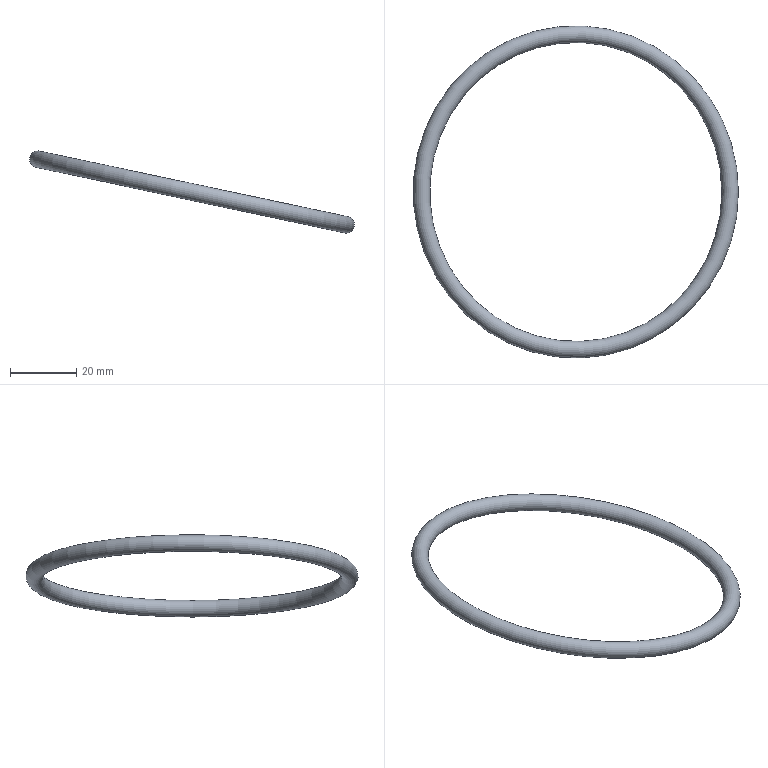Part | STEP file | 8903-010050 (O-ring) | 1 solid | 1 faces | box 97.924 x 100 x 24.752 mm | volume 5860 mm3 | torus 1
STEP:
#1=CARTESIAN_POINT('',(0.,0.,0.));
#2=DIRECTION('',(0.,0.,1.));
#3=DIRECTION('',(1.,0.,0.));
#4=AXIS2_PLACEMENT_3D('',#1,#2,#3);
#5=CARTESIAN_POINT('',(1988.852,-44.547,-308.432));
#6=VERTEX_POINT('',#5);
#7=CARTESIAN_POINT('',(1988.746,-47.045,-308.41));
#8=DIRECTION('',(-0.9772,0.04338,0.2077));
#9=DIRECTION('',(0.04243,0.9991,-0.009019));
#10=AXIS2_PLACEMENT_3D('',#7,#8,#9);
#11=CIRCLE('',#10,2.5);
#12=CARTESIAN_POINT('',(1986.73,-94.5,-307.981));
#13=DIRECTION('',(-0.2079,0.,-0.9781));
#14=DIRECTION('',(0.04243,0.9991,-0.009019));
#15=AXIS2_PLACEMENT_3D('',#12,#13,#14);
#16=TOROIDAL_SURFACE('',#15,47.5,2.5);
#17=CARTESIAN_POINT('',(6.283,0.));
#18=DIRECTION('',(0.,1.));
#19=VECTOR('',#18,1.);
#20=LINE('',#17,#19);
#21=(GEOMETRIC_REPRESENTATION_CONTEXT(2)PARAMETRIC_REPRESENTATION_CONTEXT()REPRESENTATION_CONTEXT('',''));
#22=DEFINITIONAL_REPRESENTATION('',(#20),#21);
#23=PCURVE('',#16,#22);
#24=CARTESIAN_POINT('',(0.,0.));
#25=DIRECTION('',(0.,1.));
#26=VECTOR('',#25,1.);
#27=LINE('',#24,#26);
#28=(GEOMETRIC_REPRESENTATION_CONTEXT(2)PARAMETRIC_REPRESENTATION_CONTEXT()REPRESENTATION_CONTEXT('',''));
#29=DEFINITIONAL_REPRESENTATION('',(#27),#28);
#30=PCURVE('',#16,#29);
#31=SEAM_CURVE('',#11,(#23,#30),.PCURVE_S1.);
#32=EDGE_CURVE('',#6,#6,#31,.T.);
#33=ORIENTED_EDGE('',*,*,#32,.T.);
#34=CARTESIAN_POINT('',(1986.73,-94.5,-307.981));
#35=DIRECTION('',(0.2079,0.,0.9781));
#36=DIRECTION('',(0.04243,0.9991,-0.009019));
#37=AXIS2_PLACEMENT_3D('',#34,#35,#36);
#38=CIRCLE('',#37,50.);
#39=CARTESIAN_POINT('',(6.283,6.283));
#40=DIRECTION('',(-1.,0.));
#41=VECTOR('',#40,1.);
#42=LINE('',#39,#41);
#43=(GEOMETRIC_REPRESENTATION_CONTEXT(2)PARAMETRIC_REPRESENTATION_CONTEXT()REPRESENTATION_CONTEXT('',''));
#44=DEFINITIONAL_REPRESENTATION('',(#42),#43);
#45=PCURVE('',#16,#44);
#46=CARTESIAN_POINT('',(6.283,0.));
#47=DIRECTION('',(-1.,0.));
#48=VECTOR('',#47,1.);
#49=LINE('',#46,#48);
#50=(GEOMETRIC_REPRESENTATION_CONTEXT(2)PARAMETRIC_REPRESENTATION_CONTEXT()REPRESENTATION_CONTEXT('',''));
#51=DEFINITIONAL_REPRESENTATION('',(#49),#50);
#52=PCURVE('',#16,#51);
#53=SEAM_CURVE('',#38,(#45,#52),.PCURVE_S1.);
#54=EDGE_CURVE('',#6,#6,#53,.T.);
#55=ORIENTED_EDGE('',*,*,#54,.T.);
#56=ORIENTED_EDGE('',*,*,#32,.F.);
#57=ORIENTED_EDGE('',*,*,#54,.F.);
#58=EDGE_LOOP('',(#33,#55,#56,#57));
#59=FACE_BOUND('',#58,.T.);
#60=ADVANCED_FACE('',(#59),#16,.T.);
#61=CLOSED_SHELL('',(#60));
#62=MANIFOLD_SOLID_BREP('',#61);
#63=(LENGTH_UNIT()NAMED_UNIT(*)SI_UNIT(.MILLI.,.METRE.));
#64=UNCERTAINTY_MEASURE_WITH_UNIT(LENGTH_MEASURE(0.0000001),#63,'','');
#65=(NAMED_UNIT(*)PLANE_ANGLE_UNIT()SI_UNIT($,.RADIAN.));
#66=(NAMED_UNIT(*)SI_UNIT($,.STERADIAN.)SOLID_ANGLE_UNIT());
#67=(GEOMETRIC_REPRESENTATION_CONTEXT(3)GLOBAL_UNCERTAINTY_ASSIGNED_CONTEXT((#64))GLOBAL_UNIT_ASSIGNED_CONTEXT((#63,#65,#66))REPRESENTATION_CONTEXT('',''));
#68=ADVANCED_BREP_SHAPE_REPRESENTATION('',(#4,#62),#67);